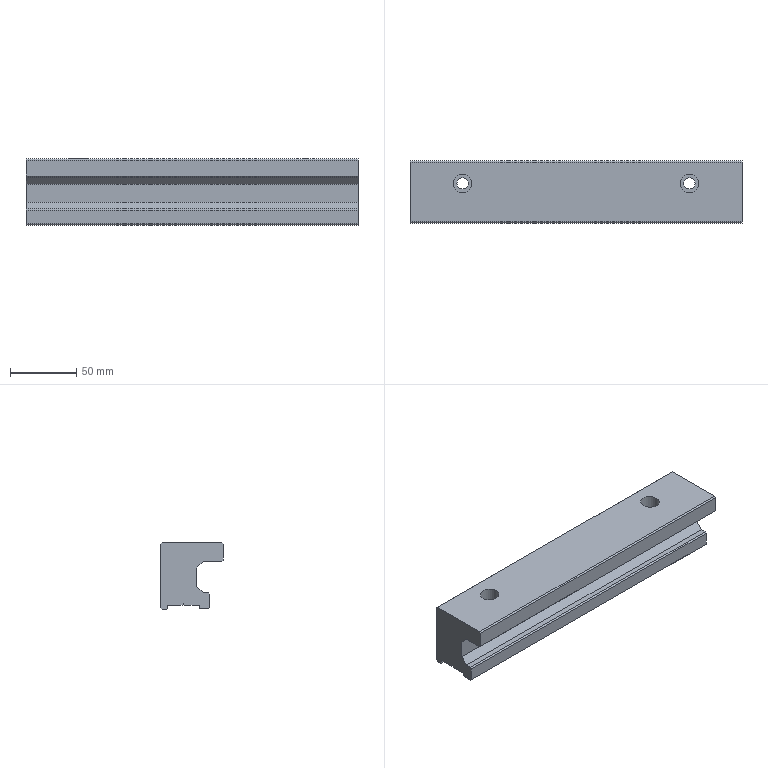Part | NX | features EXTRUDE 3, DATUM_CSYS 2, SKETCH 1 | 1 solid | 37 faces | box 250 x 47 x 50 mm | volume 417029 mm3 | plane 33 | cylinder 4 | commonest cylinder face diameters 8.5 x2 14 x2
STEP:
#1=CARTESIAN_POINT('',(5325.419,6882.013,-47.));
#2=VERTEX_POINT('',#1);
#3=CARTESIAN_POINT('',(5317.158,6882.013,-47.));
#4=VERTEX_POINT('',#3);
#5=CARTESIAN_POINT('',(5321.289,6883.013,-47.));
#6=DIRECTION('',(0.,0.,1.));
#7=DIRECTION('',(1.,0.,0.));
#8=AXIS2_PLACEMENT_3D('',#5,#6,#7);
#9=CIRCLE('',#8,4.25);
#10=EDGE_CURVE('',#2,#4,#9,.F.);
#11=ORIENTED_EDGE('',*,*,#10,.T.);
#12=CARTESIAN_POINT('',(5317.039,6883.013,-46.));
#13=VERTEX_POINT('',#12);
#14=CARTESIAN_POINT('',(5321.289,6883.013,-46.));
#15=DIRECTION('',(0.,-0.7071,0.7071));
#16=DIRECTION('',(0.,0.7071,0.7071));
#17=AXIS2_PLACEMENT_3D('',#14,#15,#16);
#18=ELLIPSE('',#17,6.01,4.25);
#19=EDGE_CURVE('',#4,#13,#18,.F.);
#20=ORIENTED_EDGE('',*,*,#19,.T.);
#21=CARTESIAN_POINT('',(5317.158,6884.013,-47.));
#22=VERTEX_POINT('',#21);
#23=CARTESIAN_POINT('',(5321.289,6883.013,-46.));
#24=DIRECTION('',(0.,0.7071,0.7071));
#25=DIRECTION('',(0.,-0.7071,0.7071));
#26=AXIS2_PLACEMENT_3D('',#23,#24,#25);
#27=ELLIPSE('',#26,6.01,4.25);
#28=EDGE_CURVE('',#13,#22,#27,.F.);
#29=ORIENTED_EDGE('',*,*,#28,.T.);
#30=CARTESIAN_POINT('',(5325.419,6884.013,-47.));
#31=VERTEX_POINT('',#30);
#32=CARTESIAN_POINT('',(5321.289,6883.013,-47.));
#33=DIRECTION('',(0.,0.,1.));
#34=DIRECTION('',(1.,0.,0.));
#35=AXIS2_PLACEMENT_3D('',#32,#33,#34);
#36=CIRCLE('',#35,4.25);
#37=EDGE_CURVE('',#22,#31,#36,.F.);
#38=ORIENTED_EDGE('',*,*,#37,.T.);
#39=CARTESIAN_POINT('',(5325.539,6883.013,-46.));
#40=VERTEX_POINT('',#39);
#41=CARTESIAN_POINT('',(5321.289,6883.013,-46.));
#42=DIRECTION('',(0.,0.7071,0.7071));
#43=DIRECTION('',(0.,-0.7071,0.7071));
#44=AXIS2_PLACEMENT_3D('',#41,#42,#43);
#45=ELLIPSE('',#44,6.01,4.25);
#46=EDGE_CURVE('',#31,#40,#45,.F.);
#47=ORIENTED_EDGE('',*,*,#46,.T.);
#48=CARTESIAN_POINT('',(5321.289,6883.013,-46.));
#49=DIRECTION('',(0.,-0.7071,0.7071));
#50=DIRECTION('',(0.,0.7071,0.7071));
#51=AXIS2_PLACEMENT_3D('',#48,#49,#50);
#52=ELLIPSE('',#51,6.01,4.25);
#53=EDGE_CURVE('',#40,#2,#52,.F.);
#54=ORIENTED_EDGE('',*,*,#53,.T.);
#55=EDGE_LOOP('',(#11,#20,#29,#38,#47,#54));
#56=FACE_BOUND('',#55,.T.);
#57=CARTESIAN_POINT('',(5325.539,6883.013,-12.));
#58=VERTEX_POINT('',#57);
#59=CARTESIAN_POINT('',(5321.289,6883.013,-12.));
#60=DIRECTION('',(0.,0.,1.));
#61=DIRECTION('',(1.,0.,0.));
#62=AXIS2_PLACEMENT_3D('',#59,#60,#61);
#63=CIRCLE('',#62,4.25);
#64=EDGE_CURVE('',#58,#58,#63,.F.);
#65=ORIENTED_EDGE('',*,*,#64,.F.);
#66=EDGE_LOOP('',(#65));
#67=FACE_BOUND('',#66,.T.);
#68=CARTESIAN_POINT('',(5321.289,6883.013,-55000.));
#69=DIRECTION('',(0.,0.,1.));
#70=DIRECTION('',(1.,0.,0.));
#71=AXIS2_PLACEMENT_3D('',#68,#69,#70);
#72=CYLINDRICAL_SURFACE('',#71,4.25);
#73=ADVANCED_FACE('',(#56,#67),#72,.F.);
#74=CARTESIAN_POINT('',(5496.279,6882.013,-47.));
#75=VERTEX_POINT('',#74);
#76=CARTESIAN_POINT('',(5488.017,6882.013,-47.));
#77=VERTEX_POINT('',#76);
#78=CARTESIAN_POINT('',(5492.148,6883.013,-47.));
#79=DIRECTION('',(0.,0.,1.));
#80=DIRECTION('',(1.,0.,0.));
#81=AXIS2_PLACEMENT_3D('',#78,#79,#80);
#82=CIRCLE('',#81,4.25);
#83=EDGE_CURVE('',#75,#77,#82,.F.);
#84=ORIENTED_EDGE('',*,*,#83,.T.);
#85=CARTESIAN_POINT('',(5487.898,6883.013,-46.));
#86=VERTEX_POINT('',#85);
#87=CARTESIAN_POINT('',(5492.148,6883.013,-46.));
#88=DIRECTION('',(0.,-0.7071,0.7071));
#89=DIRECTION('',(0.,0.7071,0.7071));
#90=AXIS2_PLACEMENT_3D('',#87,#88,#89);
#91=ELLIPSE('',#90,6.01,4.25);
#92=EDGE_CURVE('',#77,#86,#91,.F.);
#93=ORIENTED_EDGE('',*,*,#92,.T.);
#94=CARTESIAN_POINT('',(5488.017,6884.013,-47.));
#95=VERTEX_POINT('',#94);
#96=CARTESIAN_POINT('',(5492.148,6883.013,-46.));
#97=DIRECTION('',(0.,0.7071,0.7071));
#98=DIRECTION('',(0.,-0.7071,0.7071));
#99=AXIS2_PLACEMENT_3D('',#96,#97,#98);
#100=ELLIPSE('',#99,6.01,4.25);
#101=EDGE_CURVE('',#86,#95,#100,.F.);
#102=ORIENTED_EDGE('',*,*,#101,.T.);
#103=CARTESIAN_POINT('',(5496.279,6884.013,-47.));
#104=VERTEX_POINT('',#103);
#105=CARTESIAN_POINT('',(5492.148,6883.013,-47.));
#106=DIRECTION('',(0.,0.,1.));
#107=DIRECTION('',(1.,0.,0.));
#108=AXIS2_PLACEMENT_3D('',#105,#106,#107);
#109=CIRCLE('',#108,4.25);
#110=EDGE_CURVE('',#95,#104,#109,.F.);
#111=ORIENTED_EDGE('',*,*,#110,.T.);
#112=CARTESIAN_POINT('',(5496.398,6883.013,-46.));
#113=VERTEX_POINT('',#112);
#114=CARTESIAN_POINT('',(5492.148,6883.013,-46.));
#115=DIRECTION('',(0.,0.7071,0.7071));
#116=DIRECTION('',(0.,-0.7071,0.7071));
#117=AXIS2_PLACEMENT_3D('',#114,#115,#116);
#118=ELLIPSE('',#117,6.01,4.25);
#119=EDGE_CURVE('',#104,#113,#118,.F.);
#120=ORIENTED_EDGE('',*,*,#119,.T.);
#121=CARTESIAN_POINT('',(5492.148,6883.013,-46.));
#122=DIRECTION('',(0.,-0.7071,0.7071));
#123=DIRECTION('',(0.,0.7071,0.7071));
#124=AXIS2_PLACEMENT_3D('',#121,#122,#123);
#125=ELLIPSE('',#124,6.01,4.25);
#126=EDGE_CURVE('',#113,#75,#125,.F.);
#127=ORIENTED_EDGE('',*,*,#126,.T.);
#128=EDGE_LOOP('',(#84,#93,#102,#111,#120,#127));
#129=FACE_BOUND('',#128,.T.);
#130=CARTESIAN_POINT('',(5496.398,6883.013,-12.));
#131=VERTEX_POINT('',#130);
#132=CARTESIAN_POINT('',(5492.148,6883.013,-12.));
#133=DIRECTION('',(0.,0.,1.));
#134=DIRECTION('',(1.,0.,0.));
#135=AXIS2_PLACEMENT_3D('',#132,#133,#134);
#136=CIRCLE('',#135,4.25);
#137=EDGE_CURVE('',#131,#131,#136,.F.);
#138=ORIENTED_EDGE('',*,*,#137,.F.);
#139=EDGE_LOOP('',(#138));
#140=FACE_BOUND('',#139,.T.);
#141=CARTESIAN_POINT('',(5492.148,6883.013,-55000.));
#142=DIRECTION('',(0.,0.,1.));
#143=DIRECTION('',(1.,0.,0.));
#144=AXIS2_PLACEMENT_3D('',#141,#142,#143);
#145=CYLINDRICAL_SURFACE('',#144,4.25);
#146=ADVANCED_FACE('',(#129,#140),#145,.F.);
#147=ORIENTED_EDGE('',*,*,#110,.F.);
#148=CARTESIAN_POINT('',(5281.718,6884.013,-47.));
#149=DIRECTION('',(1.,0.,0.));
#150=VECTOR('',#149,1000.);
#151=LINE('',#148,#150);
#152=EDGE_CURVE('',#31,#95,#151,.T.);
#153=ORIENTED_EDGE('',*,*,#152,.F.);
#154=ORIENTED_EDGE('',*,*,#37,.F.);
#155=CARTESIAN_POINT('',(5281.718,6884.013,-47.));
#156=VERTEX_POINT('',#155);
#157=CARTESIAN_POINT('',(5281.718,6884.013,-47.));
#158=DIRECTION('',(1.,0.,0.));
#159=VECTOR('',#158,1000.);
#160=LINE('',#157,#159);
#161=EDGE_CURVE('',#156,#22,#160,.T.);
#162=ORIENTED_EDGE('',*,*,#161,.F.);
#163=CARTESIAN_POINT('',(5281.718,6895.088,-47.));
#164=VERTEX_POINT('',#163);
#165=CARTESIAN_POINT('',(5281.718,6895.088,-47.));
#166=DIRECTION('',(0.,-1.,0.));
#167=VECTOR('',#166,1000.);
#168=LINE('',#165,#167);
#169=EDGE_CURVE('',#164,#156,#168,.T.);
#170=ORIENTED_EDGE('',*,*,#169,.F.);
#171=CARTESIAN_POINT('',(5531.718,6895.088,-47.));
#172=VERTEX_POINT('',#171);
#173=CARTESIAN_POINT('',(5281.718,6895.088,-47.));
#174=DIRECTION('',(1.,0.,0.));
#175=VECTOR('',#174,1000.);
#176=LINE('',#173,#175);
#177=EDGE_CURVE('',#164,#172,#176,.T.);
#178=ORIENTED_EDGE('',*,*,#177,.T.);
#179=CARTESIAN_POINT('',(5531.718,6884.013,-47.));
#180=VERTEX_POINT('',#179);
#181=CARTESIAN_POINT('',(5531.718,6895.088,-47.));
#182=DIRECTION('',(0.,-1.,0.));
#183=VECTOR('',#182,1000.);
#184=LINE('',#181,#183);
#185=EDGE_CURVE('',#172,#180,#184,.T.);
#186=ORIENTED_EDGE('',*,*,#185,.T.);
#187=CARTESIAN_POINT('',(5281.718,6884.013,-47.));
#188=DIRECTION('',(1.,0.,0.));
#189=VECTOR('',#188,1000.);
#190=LINE('',#187,#189);
#191=EDGE_CURVE('',#104,#180,#190,.T.);
#192=ORIENTED_EDGE('',*,*,#191,.F.);
#193=EDGE_LOOP('',(#147,#153,#154,#162,#170,#178,#186,#192));
#194=FACE_BOUND('',#193,.T.);
#195=CARTESIAN_POINT('',(5281.718,6895.088,-47.));
#196=DIRECTION('',(0.,0.,1.));
#197=DIRECTION('',(1.,0.,0.));
#198=AXIS2_PLACEMENT_3D('',#195,#196,#197);
#199=PLANE('',#198);
#200=ADVANCED_FACE('',(#194),#199,.F.);
#201=ORIENTED_EDGE('',*,*,#101,.F.);
#202=CARTESIAN_POINT('',(5281.718,6883.013,-46.));
#203=DIRECTION('',(1.,0.,0.));
#204=VECTOR('',#203,1000.);
#205=LINE('',#202,#204);
#206=EDGE_CURVE('',#40,#86,#205,.T.);
#207=ORIENTED_EDGE('',*,*,#206,.F.);
#208=ORIENTED_EDGE('',*,*,#46,.F.);
#209=ORIENTED_EDGE('',*,*,#152,.T.);
#210=EDGE_LOOP('',(#201,#207,#208,#209));
#211=FACE_BOUND('',#210,.T.);
#212=CARTESIAN_POINT('',(5281.718,6884.013,-47.));
#213=DIRECTION('',(0.,0.7071,0.7071));
#214=DIRECTION('',(0.,-0.7071,0.7071));
#215=AXIS2_PLACEMENT_3D('',#212,#213,#214);
#216=PLANE('',#215);
#217=ADVANCED_FACE('',(#211),#216,.F.);
#218=ORIENTED_EDGE('',*,*,#119,.F.);
#219=ORIENTED_EDGE('',*,*,#191,.T.);
#220=CARTESIAN_POINT('',(5531.718,6883.013,-46.));
#221=VERTEX_POINT('',#220);
#222=CARTESIAN_POINT('',(5531.718,6884.013,-47.));
#223=DIRECTION('',(0.,-0.7071,0.7071));
#224=VECTOR('',#223,1000.);
#225=LINE('',#222,#224);
#226=EDGE_CURVE('',#180,#221,#225,.T.);
#227=ORIENTED_EDGE('',*,*,#226,.T.);
#228=CARTESIAN_POINT('',(5281.718,6883.013,-46.));
#229=DIRECTION('',(1.,0.,0.));
#230=VECTOR('',#229,1000.);
#231=LINE('',#228,#230);
#232=EDGE_CURVE('',#113,#221,#231,.T.);
#233=ORIENTED_EDGE('',*,*,#232,.F.);
#234=EDGE_LOOP('',(#218,#219,#227,#233));
#235=FACE_BOUND('',#234,.T.);
#236=CARTESIAN_POINT('',(5281.718,6884.013,-47.));
#237=DIRECTION('',(0.,0.7071,0.7071));
#238=DIRECTION('',(0.,-0.7071,0.7071));
#239=AXIS2_PLACEMENT_3D('',#236,#237,#238);
#240=PLANE('',#239);
#241=ADVANCED_FACE('',(#235),#240,.F.);
#242=ORIENTED_EDGE('',*,*,#28,.F.);
#243=CARTESIAN_POINT('',(5281.718,6883.013,-46.));
#244=VERTEX_POINT('',#243);
#245=CARTESIAN_POINT('',(5281.718,6883.013,-46.));
#246=DIRECTION('',(1.,0.,0.));
#247=VECTOR('',#246,1000.);
#248=LINE('',#245,#247);
#249=EDGE_CURVE('',#244,#13,#248,.T.);
#250=ORIENTED_EDGE('',*,*,#249,.F.);
#251=CARTESIAN_POINT('',(5281.718,6884.013,-47.));
#252=DIRECTION('',(0.,-0.7071,0.7071));
#253=VECTOR('',#252,1000.);
#254=LINE('',#251,#253);
#255=EDGE_CURVE('',#156,#244,#254,.T.);
#256=ORIENTED_EDGE('',*,*,#255,.F.);
#257=ORIENTED_EDGE('',*,*,#161,.T.);
#258=EDGE_LOOP('',(#242,#250,#256,#257));
#259=FACE_BOUND('',#258,.T.);
#260=CARTESIAN_POINT('',(5281.718,6884.013,-47.));
#261=DIRECTION('',(0.,0.7071,0.7071));
#262=DIRECTION('',(0.,-0.7071,0.7071));
#263=AXIS2_PLACEMENT_3D('',#260,#261,#262);
#264=PLANE('',#263);
#265=ADVANCED_FACE('',(#259),#264,.F.);
#266=ORIENTED_EDGE('',*,*,#126,.F.);
#267=ORIENTED_EDGE('',*,*,#232,.T.);
#268=CARTESIAN_POINT('',(5531.718,6882.013,-47.));
#269=VERTEX_POINT('',#268);
#270=CARTESIAN_POINT('',(5531.718,6883.013,-46.));
#271=DIRECTION('',(0.,-0.7071,-0.7071));
#272=VECTOR('',#271,1000.);
#273=LINE('',#270,#272);
#274=EDGE_CURVE('',#221,#269,#273,.T.);
#275=ORIENTED_EDGE('',*,*,#274,.T.);
#276=CARTESIAN_POINT('',(5281.718,6882.013,-47.));
#277=DIRECTION('',(1.,0.,0.));
#278=VECTOR('',#277,1000.);
#279=LINE('',#276,#278);
#280=EDGE_CURVE('',#75,#269,#279,.T.);
#281=ORIENTED_EDGE('',*,*,#280,.F.);
#282=EDGE_LOOP('',(#266,#267,#275,#281));
#283=FACE_BOUND('',#282,.T.);
#284=CARTESIAN_POINT('',(5281.718,6883.013,-46.));
#285=DIRECTION('',(0.,-0.7071,0.7071));
#286=DIRECTION('',(0.,-0.7071,-0.7071));
#287=AXIS2_PLACEMENT_3D('',#284,#285,#286);
#288=PLANE('',#287);
#289=ADVANCED_FACE('',(#283),#288,.F.);
#290=ORIENTED_EDGE('',*,*,#92,.F.);
#291=CARTESIAN_POINT('',(5281.718,6882.013,-47.));
#292=DIRECTION('',(1.,0.,0.));
#293=VECTOR('',#292,1000.);
#294=LINE('',#291,#293);
#295=EDGE_CURVE('',#2,#77,#294,.T.);
#296=ORIENTED_EDGE('',*,*,#295,.F.);
#297=ORIENTED_EDGE('',*,*,#53,.F.);
#298=ORIENTED_EDGE('',*,*,#206,.T.);
#299=EDGE_LOOP('',(#290,#296,#297,#298));
#300=FACE_BOUND('',#299,.T.);
#301=CARTESIAN_POINT('',(5281.718,6883.013,-46.));
#302=DIRECTION('',(0.,-0.7071,0.7071));
#303=DIRECTION('',(0.,-0.7071,-0.7071));
#304=AXIS2_PLACEMENT_3D('',#301,#302,#303);
#305=PLANE('',#304);
#306=ADVANCED_FACE('',(#300),#305,.F.);
#307=ORIENTED_EDGE('',*,*,#19,.F.);
#308=CARTESIAN_POINT('',(5281.718,6882.013,-47.));
#309=VERTEX_POINT('',#308);
#310=CARTESIAN_POINT('',(5281.718,6882.013,-47.));
#311=DIRECTION('',(1.,0.,0.));
#312=VECTOR('',#311,1000.);
#313=LINE('',#310,#312);
#314=EDGE_CURVE('',#309,#4,#313,.T.);
#315=ORIENTED_EDGE('',*,*,#314,.F.);
#316=CARTESIAN_POINT('',(5281.718,6883.013,-46.));
#317=DIRECTION('',(0.,-0.7071,-0.7071));
#318=VECTOR('',#317,1000.);
#319=LINE('',#316,#318);
#320=EDGE_CURVE('',#244,#309,#319,.T.);
#321=ORIENTED_EDGE('',*,*,#320,.F.);
#322=ORIENTED_EDGE('',*,*,#249,.T.);
#323=EDGE_LOOP('',(#307,#315,#321,#322));
#324=FACE_BOUND('',#323,.T.);
#325=CARTESIAN_POINT('',(5281.718,6883.013,-46.));
#326=DIRECTION('',(0.,-0.7071,0.7071));
#327=DIRECTION('',(0.,-0.7071,-0.7071));
#328=AXIS2_PLACEMENT_3D('',#325,#326,#327);
#329=PLANE('',#328);
#330=ADVANCED_FACE('',(#324),#329,.F.);
#331=ORIENTED_EDGE('',*,*,#83,.F.);
#332=ORIENTED_EDGE('',*,*,#280,.T.);
#333=CARTESIAN_POINT('',(5531.718,6870.938,-47.));
#334=VERTEX_POINT('',#333);
#335=CARTESIAN_POINT('',(5531.718,6882.013,-47.));
#336=DIRECTION('',(0.,-1.,0.));
#337=VECTOR('',#336,1000.);
#338=LINE('',#335,#337);
#339=EDGE_CURVE('',#269,#334,#338,.T.);
#340=ORIENTED_EDGE('',*,*,#339,.T.);
#341=CARTESIAN_POINT('',(5281.718,6870.938,-47.));
#342=VERTEX_POINT('',#341);
#343=CARTESIAN_POINT('',(5281.718,6870.938,-47.));
#344=DIRECTION('',(1.,0.,0.));
#345=VECTOR('',#344,1000.);
#346=LINE('',#343,#345);
#347=EDGE_CURVE('',#342,#334,#346,.T.);
#348=ORIENTED_EDGE('',*,*,#347,.F.);
#349=CARTESIAN_POINT('',(5281.718,6882.013,-47.));
#350=DIRECTION('',(0.,-1.,0.));
#351=VECTOR('',#350,1000.);
#352=LINE('',#349,#351);
#353=EDGE_CURVE('',#309,#342,#352,.T.);
#354=ORIENTED_EDGE('',*,*,#353,.F.);
#355=ORIENTED_EDGE('',*,*,#314,.T.);
#356=ORIENTED_EDGE('',*,*,#10,.F.);
#357=ORIENTED_EDGE('',*,*,#295,.T.);
#358=EDGE_LOOP('',(#331,#332,#340,#348,#354,#355,#356,#357));
#359=FACE_BOUND('',#358,.T.);
#360=CARTESIAN_POINT('',(5281.718,6882.013,-47.));
#361=DIRECTION('',(0.,0.,1.));
#362=DIRECTION('',(1.,0.,0.));
#363=AXIS2_PLACEMENT_3D('',#360,#361,#362);
#364=PLANE('',#363);
#365=ADVANCED_FACE('',(#359),#364,.F.);
#366=CARTESIAN_POINT('',(5531.718,6899.013,0.));
#367=VERTEX_POINT('',#366);
#368=CARTESIAN_POINT('',(5531.718,6900.013,-1.));
#369=VERTEX_POINT('',#368);
#370=CARTESIAN_POINT('',(5531.718,6899.013,0.));
#371=DIRECTION('',(0.,0.7071,-0.7071));
#372=VECTOR('',#371,1000.);
#373=LINE('',#370,#372);
#374=EDGE_CURVE('',#367,#369,#373,.T.);
#375=ORIENTED_EDGE('',*,*,#374,.T.);
#376=CARTESIAN_POINT('',(5281.718,6900.013,-1.));
#377=VERTEX_POINT('',#376);
#378=CARTESIAN_POINT('',(5281.718,6900.013,-1.));
#379=DIRECTION('',(1.,0.,0.));
#380=VECTOR('',#379,1000.);
#381=LINE('',#378,#380);
#382=EDGE_CURVE('',#377,#369,#381,.T.);
#383=ORIENTED_EDGE('',*,*,#382,.F.);
#384=CARTESIAN_POINT('',(5281.718,6899.013,0.));
#385=VERTEX_POINT('',#384);
#386=CARTESIAN_POINT('',(5281.718,6899.013,0.));
#387=DIRECTION('',(0.,0.7071,-0.7071));
#388=VECTOR('',#387,1000.);
#389=LINE('',#386,#388);
#390=EDGE_CURVE('',#385,#377,#389,.T.);
#391=ORIENTED_EDGE('',*,*,#390,.F.);
#392=CARTESIAN_POINT('',(5281.718,6899.013,0.));
#393=DIRECTION('',(1.,0.,0.));
#394=VECTOR('',#393,1000.);
#395=LINE('',#392,#394);
#396=EDGE_CURVE('',#385,#367,#395,.T.);
#397=ORIENTED_EDGE('',*,*,#396,.T.);
#398=EDGE_LOOP('',(#375,#383,#391,#397));
#399=FACE_BOUND('',#398,.T.);
#400=CARTESIAN_POINT('',(5281.718,6899.013,0.));
#401=DIRECTION('',(0.,-0.7071,-0.7071));
#402=DIRECTION('',(0.,0.7071,-0.7071));
#403=AXIS2_PLACEMENT_3D('',#400,#401,#402);
#404=PLANE('',#403);
#405=ADVANCED_FACE('',(#399),#404,.F.);
#406=CARTESIAN_POINT('',(5531.718,6900.013,-49.));
#407=VERTEX_POINT('',#406);
#408=CARTESIAN_POINT('',(5531.718,6900.013,-1.));
#409=DIRECTION('',(0.,0.,-1.));
#410=VECTOR('',#409,1000.);
#411=LINE('',#408,#410);
#412=EDGE_CURVE('',#369,#407,#411,.T.);
#413=ORIENTED_EDGE('',*,*,#412,.T.);
#414=CARTESIAN_POINT('',(5281.718,6900.013,-49.));
#415=VERTEX_POINT('',#414);
#416=CARTESIAN_POINT('',(5281.718,6900.013,-49.));
#417=DIRECTION('',(1.,0.,0.));
#418=VECTOR('',#417,1000.);
#419=LINE('',#416,#418);
#420=EDGE_CURVE('',#415,#407,#419,.T.);
#421=ORIENTED_EDGE('',*,*,#420,.F.);
#422=CARTESIAN_POINT('',(5281.718,6900.013,-1.));
#423=DIRECTION('',(0.,0.,-1.));
#424=VECTOR('',#423,1000.);
#425=LINE('',#422,#424);
#426=EDGE_CURVE('',#377,#415,#425,.T.);
#427=ORIENTED_EDGE('',*,*,#426,.F.);
#428=ORIENTED_EDGE('',*,*,#382,.T.);
#429=EDGE_LOOP('',(#413,#421,#427,#428));
#430=FACE_BOUND('',#429,.T.);
#431=CARTESIAN_POINT('',(5281.718,6900.013,-1.));
#432=DIRECTION('',(0.,-1.,0.));
#433=DIRECTION('',(0.,0.,-1.));
#434=AXIS2_PLACEMENT_3D('',#431,#432,#433);
#435=PLANE('',#434);
#436=ADVANCED_FACE('',(#430),#435,.F.);
#437=CARTESIAN_POINT('',(5531.718,6899.013,-50.));
#438=VERTEX_POINT('',#437);
#439=CARTESIAN_POINT('',(5531.718,6900.013,-49.));
#440=DIRECTION('',(0.,-0.7071,-0.7071));
#441=VECTOR('',#440,1000.);
#442=LINE('',#439,#441);
#443=EDGE_CURVE('',#407,#438,#442,.T.);
#444=ORIENTED_EDGE('',*,*,#443,.T.);
#445=CARTESIAN_POINT('',(5281.718,6899.013,-50.));
#446=VERTEX_POINT('',#445);
#447=CARTESIAN_POINT('',(5281.718,6899.013,-50.));
#448=DIRECTION('',(1.,0.,0.));
#449=VECTOR('',#448,1000.);
#450=LINE('',#447,#449);
#451=EDGE_CURVE('',#446,#438,#450,.T.);
#452=ORIENTED_EDGE('',*,*,#451,.F.);
#453=CARTESIAN_POINT('',(5281.718,6900.013,-49.));
#454=DIRECTION('',(0.,-0.7071,-0.7071));
#455=VECTOR('',#454,1000.);
#456=LINE('',#453,#455);
#457=EDGE_CURVE('',#415,#446,#456,.T.);
#458=ORIENTED_EDGE('',*,*,#457,.F.);
#459=ORIENTED_EDGE('',*,*,#420,.T.);
#460=EDGE_LOOP('',(#444,#452,#458,#459));
#461=FACE_BOUND('',#460,.T.);
#462=CARTESIAN_POINT('',(5281.718,6900.013,-49.));
#463=DIRECTION('',(0.,-0.7071,0.7071));
#464=DIRECTION('',(0.,-0.7071,-0.7071));
#465=AXIS2_PLACEMENT_3D('',#462,#463,#464);
#466=PLANE('',#465);
#467=ADVANCED_FACE('',(#461),#466,.F.);
#468=CARTESIAN_POINT('',(5531.718,6895.588,-50.));
#469=VERTEX_POINT('',#468);
#470=CARTESIAN_POINT('',(5531.718,6899.013,-50.));
#471=DIRECTION('',(0.,-1.,0.));
#472=VECTOR('',#471,1000.);
#473=LINE('',#470,#472);
#474=EDGE_CURVE('',#438,#469,#473,.T.);
#475=ORIENTED_EDGE('',*,*,#474,.T.);
#476=CARTESIAN_POINT('',(5281.718,6895.588,-50.));
#477=VERTEX_POINT('',#476);
#478=CARTESIAN_POINT('',(5281.718,6895.588,-50.));
#479=DIRECTION('',(1.,0.,0.));
#480=VECTOR('',#479,1000.);
#481=LINE('',#478,#480);
#482=EDGE_CURVE('',#477,#469,#481,.T.);
#483=ORIENTED_EDGE('',*,*,#482,.F.);
#484=CARTESIAN_POINT('',(5281.718,6899.013,-50.));
#485=DIRECTION('',(0.,-1.,0.));
#486=VECTOR('',#485,1000.);
#487=LINE('',#484,#486);
#488=EDGE_CURVE('',#446,#477,#487,.T.);
#489=ORIENTED_EDGE('',*,*,#488,.F.);
#490=ORIENTED_EDGE('',*,*,#451,.T.);
#491=EDGE_LOOP('',(#475,#483,#489,#490));
#492=FACE_BOUND('',#491,.T.);
#493=CARTESIAN_POINT('',(5281.718,6899.013,-50.));
#494=DIRECTION('',(0.,0.,1.));
#495=DIRECTION('',(1.,0.,0.));
#496=AXIS2_PLACEMENT_3D('',#493,#494,#495);
#497=PLANE('',#496);
#498=ADVANCED_FACE('',(#492),#497,.F.);
#499=CARTESIAN_POINT('',(5531.718,6895.088,-49.5));
#500=VERTEX_POINT('',#499);
#501=CARTESIAN_POINT('',(5531.718,6895.588,-50.));
#502=DIRECTION('',(0.,-0.7071,0.7071));
#503=VECTOR('',#502,1000.);
#504=LINE('',#501,#503);
#505=EDGE_CURVE('',#469,#500,#504,.T.);
#506=ORIENTED_EDGE('',*,*,#505,.T.);
#507=CARTESIAN_POINT('',(5281.718,6895.088,-49.5));
#508=VERTEX_POINT('',#507);
#509=CARTESIAN_POINT('',(5281.718,6895.088,-49.5));
#510=DIRECTION('',(1.,0.,0.));
#511=VECTOR('',#510,1000.);
#512=LINE('',#509,#511);
#513=EDGE_CURVE('',#508,#500,#512,.T.);
#514=ORIENTED_EDGE('',*,*,#513,.F.);
#515=CARTESIAN_POINT('',(5281.718,6895.588,-50.));
#516=DIRECTION('',(0.,-0.7071,0.7071));
#517=VECTOR('',#516,1000.);
#518=LINE('',#515,#517);
#519=EDGE_CURVE('',#477,#508,#518,.T.);
#520=ORIENTED_EDGE('',*,*,#519,.F.);
#521=ORIENTED_EDGE('',*,*,#482,.T.);
#522=EDGE_LOOP('',(#506,#514,#520,#521));
#523=FACE_BOUND('',#522,.T.);
#524=CARTESIAN_POINT('',(5281.718,6895.588,-50.));
#525=DIRECTION('',(0.,0.7071,0.7071));
#526=DIRECTION('',(0.,-0.7071,0.7071));
#527=AXIS2_PLACEMENT_3D('',#524,#525,#526);
#528=PLANE('',#527);
#529=ADVANCED_FACE('',(#523),#528,.F.);
#530=CARTESIAN_POINT('',(5531.718,6895.088,-49.5));
#531=DIRECTION('',(0.,0.,1.));
#532=VECTOR('',#531,1000.);
#533=LINE('',#530,#532);
#534=EDGE_CURVE('',#500,#172,#533,.T.);
#535=ORIENTED_EDGE('',*,*,#534,.T.);
#536=ORIENTED_EDGE('',*,*,#177,.F.);
#537=CARTESIAN_POINT('',(5281.718,6895.088,-49.5));
#538=DIRECTION('',(0.,0.,1.));
#539=VECTOR('',#538,1000.);
#540=LINE('',#537,#539);
#541=EDGE_CURVE('',#508,#164,#540,.T.);
#542=ORIENTED_EDGE('',*,*,#541,.F.);
#543=ORIENTED_EDGE('',*,*,#513,.T.);
#544=EDGE_LOOP('',(#535,#536,#542,#543));
#545=FACE_BOUND('',#544,.T.);
#546=CARTESIAN_POINT('',(5281.718,6895.088,-49.5));
#547=DIRECTION('',(0.,1.,0.));
#548=DIRECTION('',(0.,0.,1.));
#549=AXIS2_PLACEMENT_3D('',#546,#547,#548);
#550=PLANE('',#549);
#551=ADVANCED_FACE('',(#545),#550,.F.);
#552=CARTESIAN_POINT('',(5531.718,6870.938,-49.3));
#553=VERTEX_POINT('',#552);
#554=CARTESIAN_POINT('',(5531.718,6870.938,-47.));
#555=DIRECTION('',(0.,0.,-1.));
#556=VECTOR('',#555,1000.);
#557=LINE('',#554,#556);
#558=EDGE_CURVE('',#334,#553,#557,.T.);
#559=ORIENTED_EDGE('',*,*,#558,.T.);
#560=CARTESIAN_POINT('',(5281.718,6870.938,-49.3));
#561=VERTEX_POINT('',#560);
#562=CARTESIAN_POINT('',(5281.718,6870.938,-49.3));
#563=DIRECTION('',(1.,0.,0.));
#564=VECTOR('',#563,1000.);
#565=LINE('',#562,#564);
#566=EDGE_CURVE('',#561,#553,#565,.T.);
#567=ORIENTED_EDGE('',*,*,#566,.F.);
#568=CARTESIAN_POINT('',(5281.718,6870.938,-47.));
#569=DIRECTION('',(0.,0.,-1.));
#570=VECTOR('',#569,1000.);
#571=LINE('',#568,#570);
#572=EDGE_CURVE('',#342,#561,#571,.T.);
#573=ORIENTED_EDGE('',*,*,#572,.F.);
#574=ORIENTED_EDGE('',*,*,#347,.T.);
#575=EDGE_LOOP('',(#559,#567,#573,#574));
#576=FACE_BOUND('',#575,.T.);
#577=CARTESIAN_POINT('',(5281.718,6870.938,-47.));
#578=DIRECTION('',(0.,-1.,0.));
#579=DIRECTION('',(0.,0.,-1.));
#580=AXIS2_PLACEMENT_3D('',#577,#578,#579);
#581=PLANE('',#580);
#582=ADVANCED_FACE('',(#576),#581,.F.);
#583=CARTESIAN_POINT('',(5531.718,6870.438,-49.8));
#584=VERTEX_POINT('',#583);
#585=CARTESIAN_POINT('',(5531.718,6870.938,-49.3));
#586=DIRECTION('',(0.,-0.7071,-0.7071));
#587=VECTOR('',#586,1000.);
#588=LINE('',#585,#587);
#589=EDGE_CURVE('',#553,#584,#588,.T.);
#590=ORIENTED_EDGE('',*,*,#589,.T.);
#591=CARTESIAN_POINT('',(5281.718,6870.438,-49.8));
#592=VERTEX_POINT('',#591);
#593=CARTESIAN_POINT('',(5281.718,6870.438,-49.8));
#594=DIRECTION('',(1.,0.,0.));
#595=VECTOR('',#594,1000.);
#596=LINE('',#593,#595);
#597=EDGE_CURVE('',#592,#584,#596,.T.);
#598=ORIENTED_EDGE('',*,*,#597,.F.);
#599=CARTESIAN_POINT('',(5281.718,6870.938,-49.3));
#600=DIRECTION('',(0.,-0.7071,-0.7071));
#601=VECTOR('',#600,1000.);
#602=LINE('',#599,#601);
#603=EDGE_CURVE('',#561,#592,#602,.T.);
#604=ORIENTED_EDGE('',*,*,#603,.F.);
#605=ORIENTED_EDGE('',*,*,#566,.T.);
#606=EDGE_LOOP('',(#590,#598,#604,#605));
#607=FACE_BOUND('',#606,.T.);
#608=CARTESIAN_POINT('',(5281.718,6870.938,-49.3));
#609=DIRECTION('',(0.,-0.7071,0.7071));
#610=DIRECTION('',(0.,-0.7071,-0.7071));
#611=AXIS2_PLACEMENT_3D('',#608,#609,#610);
#612=PLANE('',#611);
#613=ADVANCED_FACE('',(#607),#612,.F.);
#614=CARTESIAN_POINT('',(5531.718,6864.013,-49.8));
#615=VERTEX_POINT('',#614);
#616=CARTESIAN_POINT('',(5531.718,6870.438,-49.8));
#617=DIRECTION('',(0.,-1.,0.));
#618=VECTOR('',#617,1000.);
#619=LINE('',#616,#618);
#620=EDGE_CURVE('',#584,#615,#619,.T.);
#621=ORIENTED_EDGE('',*,*,#620,.T.);
#622=CARTESIAN_POINT('',(5281.718,6864.013,-49.8));
#623=VERTEX_POINT('',#622);
#624=CARTESIAN_POINT('',(5281.718,6864.013,-49.8));
#625=DIRECTION('',(1.,0.,0.));
#626=VECTOR('',#625,1000.);
#627=LINE('',#624,#626);
#628=EDGE_CURVE('',#623,#615,#627,.T.);
#629=ORIENTED_EDGE('',*,*,#628,.F.);
#630=CARTESIAN_POINT('',(5281.718,6870.438,-49.8));
#631=DIRECTION('',(0.,-1.,0.));
#632=VECTOR('',#631,1000.);
#633=LINE('',#630,#632);
#634=EDGE_CURVE('',#592,#623,#633,.T.);
#635=ORIENTED_EDGE('',*,*,#634,.F.);
#636=ORIENTED_EDGE('',*,*,#597,.T.);
#637=EDGE_LOOP('',(#621,#629,#635,#636));
#638=FACE_BOUND('',#637,.T.);
#639=CARTESIAN_POINT('',(5281.718,6870.438,-49.8));
#640=DIRECTION('',(0.,0.,1.));
#641=DIRECTION('',(1.,0.,0.));
#642=AXIS2_PLACEMENT_3D('',#639,#640,#641);
#643=PLANE('',#642);
#644=ADVANCED_FACE('',(#638),#643,.F.);
#645=CARTESIAN_POINT('',(5531.718,6863.013,-48.8));
#646=VERTEX_POINT('',#645);
#647=CARTESIAN_POINT('',(5531.718,6864.013,-49.8));
#648=DIRECTION('',(0.,-0.7071,0.7071));
#649=VECTOR('',#648,1000.);
#650=LINE('',#647,#649);
#651=EDGE_CURVE('',#615,#646,#650,.T.);
#652=ORIENTED_EDGE('',*,*,#651,.T.);
#653=CARTESIAN_POINT('',(5281.718,6863.013,-48.8));
#654=VERTEX_POINT('',#653);
#655=CARTESIAN_POINT('',(5281.718,6863.013,-48.8));
#656=DIRECTION('',(1.,0.,0.));
#657=VECTOR('',#656,1000.);
#658=LINE('',#655,#657);
#659=EDGE_CURVE('',#654,#646,#658,.T.);
#660=ORIENTED_EDGE('',*,*,#659,.F.);
#661=CARTESIAN_POINT('',(5281.718,6864.013,-49.8));
#662=DIRECTION('',(0.,-0.7071,0.7071));
#663=VECTOR('',#662,1000.);
#664=LINE('',#661,#663);
#665=EDGE_CURVE('',#623,#654,#664,.T.);
#666=ORIENTED_EDGE('',*,*,#665,.F.);
#667=ORIENTED_EDGE('',*,*,#628,.T.);
#668=EDGE_LOOP('',(#652,#660,#666,#667));
#669=FACE_BOUND('',#668,.T.);
#670=CARTESIAN_POINT('',(5281.718,6864.013,-49.8));
#671=DIRECTION('',(0.,0.7071,0.7071));
#672=DIRECTION('',(0.,-0.7071,0.7071));
#673=AXIS2_PLACEMENT_3D('',#670,#671,#672);
#674=PLANE('',#673);
#675=ADVANCED_FACE('',(#669),#674,.F.);
#676=CARTESIAN_POINT('',(5531.718,6863.013,-38.8));
#677=VERTEX_POINT('',#676);
#678=CARTESIAN_POINT('',(5531.718,6863.013,-48.8));
#679=DIRECTION('',(0.,0.,1.));
#680=VECTOR('',#679,1000.);
#681=LINE('',#678,#680);
#682=EDGE_CURVE('',#646,#677,#681,.T.);
#683=ORIENTED_EDGE('',*,*,#682,.T.);
#684=CARTESIAN_POINT('',(5281.718,6863.013,-38.8));
#685=VERTEX_POINT('',#684);
#686=CARTESIAN_POINT('',(5281.718,6863.013,-38.8));
#687=DIRECTION('',(1.,0.,0.));
#688=VECTOR('',#687,1000.);
#689=LINE('',#686,#688);
#690=EDGE_CURVE('',#685,#677,#689,.T.);
#691=ORIENTED_EDGE('',*,*,#690,.F.);
#692=CARTESIAN_POINT('',(5281.718,6863.013,-48.8));
#693=DIRECTION('',(0.,0.,1.));
#694=VECTOR('',#693,1000.);
#695=LINE('',#692,#694);
#696=EDGE_CURVE('',#654,#685,#695,.T.);
#697=ORIENTED_EDGE('',*,*,#696,.F.);
#698=ORIENTED_EDGE('',*,*,#659,.T.);
#699=EDGE_LOOP('',(#683,#691,#697,#698));
#700=FACE_BOUND('',#699,.T.);
#701=CARTESIAN_POINT('',(5281.718,6863.013,-48.8));
#702=DIRECTION('',(0.,1.,0.));
#703=DIRECTION('',(0.,0.,1.));
#704=AXIS2_PLACEMENT_3D('',#701,#702,#703);
#705=PLANE('',#704);
#706=ADVANCED_FACE('',(#700),#705,.F.);
#707=CARTESIAN_POINT('',(5531.718,6864.013,-37.8));
#708=VERTEX_POINT('',#707);
#709=CARTESIAN_POINT('',(5531.718,6863.013,-38.8));
#710=DIRECTION('',(0.,0.7071,0.7071));
#711=VECTOR('',#710,1000.);
#712=LINE('',#709,#711);
#713=EDGE_CURVE('',#677,#708,#712,.T.);
#714=ORIENTED_EDGE('',*,*,#713,.T.);
#715=CARTESIAN_POINT('',(5281.718,6864.013,-37.8));
#716=VERTEX_POINT('',#715);
#717=CARTESIAN_POINT('',(5281.718,6864.013,-37.8));
#718=DIRECTION('',(1.,0.,0.));
#719=VECTOR('',#718,1000.);
#720=LINE('',#717,#719);
#721=EDGE_CURVE('',#716,#708,#720,.T.);
#722=ORIENTED_EDGE('',*,*,#721,.F.);
#723=CARTESIAN_POINT('',(5281.718,6863.013,-38.8));
#724=DIRECTION('',(0.,0.7071,0.7071));
#725=VECTOR('',#724,1000.);
#726=LINE('',#723,#725);
#727=EDGE_CURVE('',#685,#716,#726,.T.);
#728=ORIENTED_EDGE('',*,*,#727,.F.);
#729=ORIENTED_EDGE('',*,*,#690,.T.);
#730=EDGE_LOOP('',(#714,#722,#728,#729));
#731=FACE_BOUND('',#730,.T.);
#732=CARTESIAN_POINT('',(5281.718,6863.013,-38.8));
#733=DIRECTION('',(0.,0.7071,-0.7071));
#734=DIRECTION('',(0.,0.7071,0.7071));
#735=AXIS2_PLACEMENT_3D('',#732,#733,#734);
#736=PLANE('',#735);
#737=ADVANCED_FACE('',(#731),#736,.F.);
#738=CARTESIAN_POINT('',(5531.718,6868.013,-37.8));
#739=VERTEX_POINT('',#738);
#740=CARTESIAN_POINT('',(5531.718,6864.013,-37.8));
#741=DIRECTION('',(0.,1.,0.));
#742=VECTOR('',#741,1000.);
#743=LINE('',#740,#742);
#744=EDGE_CURVE('',#708,#739,#743,.T.);
#745=ORIENTED_EDGE('',*,*,#744,.T.);
#746=CARTESIAN_POINT('',(5281.718,6868.013,-37.8));
#747=VERTEX_POINT('',#746);
#748=CARTESIAN_POINT('',(5281.718,6868.013,-37.8));
#749=DIRECTION('',(1.,0.,0.));
#750=VECTOR('',#749,1000.);
#751=LINE('',#748,#750);
#752=EDGE_CURVE('',#747,#739,#751,.T.);
#753=ORIENTED_EDGE('',*,*,#752,.F.);
#754=CARTESIAN_POINT('',(5281.718,6864.013,-37.8));
#755=DIRECTION('',(0.,1.,0.));
#756=VECTOR('',#755,1000.);
#757=LINE('',#754,#756);
#758=EDGE_CURVE('',#716,#747,#757,.T.);
#759=ORIENTED_EDGE('',*,*,#758,.F.);
#760=ORIENTED_EDGE('',*,*,#721,.T.);
#761=EDGE_LOOP('',(#745,#753,#759,#760));
#762=FACE_BOUND('',#761,.T.);
#763=CARTESIAN_POINT('',(5281.718,6864.013,-37.8));
#764=DIRECTION('',(0.,0.,-1.));
#765=DIRECTION('',(-1.,0.,0.));
#766=AXIS2_PLACEMENT_3D('',#763,#764,#765);
#767=PLANE('',#766);
#768=ADVANCED_FACE('',(#762),#767,.F.);
#769=CARTESIAN_POINT('',(5531.718,6873.013,-32.8));
#770=VERTEX_POINT('',#769);
#771=CARTESIAN_POINT('',(5531.718,6868.013,-37.8));
#772=DIRECTION('',(0.,0.7071,0.7071));
#773=VECTOR('',#772,1000.);
#774=LINE('',#771,#773);
#775=EDGE_CURVE('',#739,#770,#774,.T.);
#776=ORIENTED_EDGE('',*,*,#775,.T.);
#777=CARTESIAN_POINT('',(5281.718,6873.013,-32.8));
#778=VERTEX_POINT('',#777);
#779=CARTESIAN_POINT('',(5281.718,6873.013,-32.8));
#780=DIRECTION('',(1.,0.,0.));
#781=VECTOR('',#780,1000.);
#782=LINE('',#779,#781);
#783=EDGE_CURVE('',#778,#770,#782,.T.);
#784=ORIENTED_EDGE('',*,*,#783,.F.);
#785=CARTESIAN_POINT('',(5281.718,6868.013,-37.8));
#786=DIRECTION('',(0.,0.7071,0.7071));
#787=VECTOR('',#786,1000.);
#788=LINE('',#785,#787);
#789=EDGE_CURVE('',#747,#778,#788,.T.);
#790=ORIENTED_EDGE('',*,*,#789,.F.);
#791=ORIENTED_EDGE('',*,*,#752,.T.);
#792=EDGE_LOOP('',(#776,#784,#790,#791));
#793=FACE_BOUND('',#792,.T.);
#794=CARTESIAN_POINT('',(5281.718,6868.013,-37.8));
#795=DIRECTION('',(0.,0.7071,-0.7071));
#796=DIRECTION('',(0.,0.7071,0.7071));
#797=AXIS2_PLACEMENT_3D('',#794,#795,#796);
#798=PLANE('',#797);
#799=ADVANCED_FACE('',(#793),#798,.F.);
#800=CARTESIAN_POINT('',(5531.718,6873.013,-19.));
#801=VERTEX_POINT('',#800);
#802=CARTESIAN_POINT('',(5531.718,6873.013,-32.8));
#803=DIRECTION('',(0.,0.,1.));
#804=VECTOR('',#803,1000.);
#805=LINE('',#802,#804);
#806=EDGE_CURVE('',#770,#801,#805,.T.);
#807=ORIENTED_EDGE('',*,*,#806,.T.);
#808=CARTESIAN_POINT('',(5281.718,6873.013,-19.));
#809=VERTEX_POINT('',#808);
#810=CARTESIAN_POINT('',(5281.718,6873.013,-19.));
#811=DIRECTION('',(1.,0.,0.));
#812=VECTOR('',#811,1000.);
#813=LINE('',#810,#812);
#814=EDGE_CURVE('',#809,#801,#813,.T.);
#815=ORIENTED_EDGE('',*,*,#814,.F.);
#816=CARTESIAN_POINT('',(5281.718,6873.013,-32.8));
#817=DIRECTION('',(0.,0.,1.));
#818=VECTOR('',#817,1000.);
#819=LINE('',#816,#818);
#820=EDGE_CURVE('',#778,#809,#819,.T.);
#821=ORIENTED_EDGE('',*,*,#820,.F.);
#822=ORIENTED_EDGE('',*,*,#783,.T.);
#823=EDGE_LOOP('',(#807,#815,#821,#822));
#824=FACE_BOUND('',#823,.T.);
#825=CARTESIAN_POINT('',(5281.718,6873.013,-32.8));
#826=DIRECTION('',(0.,1.,0.));
#827=DIRECTION('',(0.,0.,1.));
#828=AXIS2_PLACEMENT_3D('',#825,#826,#827);
#829=PLANE('',#828);
#830=ADVANCED_FACE('',(#824),#829,.F.);
#831=CARTESIAN_POINT('',(5531.718,6868.013,-14.));
#832=VERTEX_POINT('',#831);
#833=CARTESIAN_POINT('',(5531.718,6873.013,-19.));
#834=DIRECTION('',(0.,-0.7071,0.7071));
#835=VECTOR('',#834,1000.);
#836=LINE('',#833,#835);
#837=EDGE_CURVE('',#801,#832,#836,.T.);
#838=ORIENTED_EDGE('',*,*,#837,.T.);
#839=CARTESIAN_POINT('',(5281.718,6868.013,-14.));
#840=VERTEX_POINT('',#839);
#841=CARTESIAN_POINT('',(5281.718,6868.013,-14.));
#842=DIRECTION('',(1.,0.,0.));
#843=VECTOR('',#842,1000.);
#844=LINE('',#841,#843);
#845=EDGE_CURVE('',#840,#832,#844,.T.);
#846=ORIENTED_EDGE('',*,*,#845,.F.);
#847=CARTESIAN_POINT('',(5281.718,6873.013,-19.));
#848=DIRECTION('',(0.,-0.7071,0.7071));
#849=VECTOR('',#848,1000.);
#850=LINE('',#847,#849);
#851=EDGE_CURVE('',#809,#840,#850,.T.);
#852=ORIENTED_EDGE('',*,*,#851,.F.);
#853=ORIENTED_EDGE('',*,*,#814,.T.);
#854=EDGE_LOOP('',(#838,#846,#852,#853));
#855=FACE_BOUND('',#854,.T.);
#856=CARTESIAN_POINT('',(5281.718,6873.013,-19.));
#857=DIRECTION('',(0.,0.7071,0.7071));
#858=DIRECTION('',(0.,-0.7071,0.7071));
#859=AXIS2_PLACEMENT_3D('',#856,#857,#858);
#860=PLANE('',#859);
#861=ADVANCED_FACE('',(#855),#860,.F.);
#862=CARTESIAN_POINT('',(5531.718,6854.013,-14.));
#863=VERTEX_POINT('',#862);
#864=CARTESIAN_POINT('',(5531.718,6868.013,-14.));
#865=DIRECTION('',(0.,-1.,0.));
#866=VECTOR('',#865,1000.);
#867=LINE('',#864,#866);
#868=EDGE_CURVE('',#832,#863,#867,.T.);
#869=ORIENTED_EDGE('',*,*,#868,.T.);
#870=CARTESIAN_POINT('',(5281.718,6854.013,-14.));
#871=VERTEX_POINT('',#870);
#872=CARTESIAN_POINT('',(5281.718,6854.013,-14.));
#873=DIRECTION('',(1.,0.,0.));
#874=VECTOR('',#873,1000.);
#875=LINE('',#872,#874);
#876=EDGE_CURVE('',#871,#863,#875,.T.);
#877=ORIENTED_EDGE('',*,*,#876,.F.);
#878=CARTESIAN_POINT('',(5281.718,6868.013,-14.));
#879=DIRECTION('',(0.,-1.,0.));
#880=VECTOR('',#879,1000.);
#881=LINE('',#878,#880);
#882=EDGE_CURVE('',#840,#871,#881,.T.);
#883=ORIENTED_EDGE('',*,*,#882,.F.);
#884=ORIENTED_EDGE('',*,*,#845,.T.);
#885=EDGE_LOOP('',(#869,#877,#883,#884));
#886=FACE_BOUND('',#885,.T.);
#887=CARTESIAN_POINT('',(5281.718,6868.013,-14.));
#888=DIRECTION('',(0.,0.,1.));
#889=DIRECTION('',(1.,0.,0.));
#890=AXIS2_PLACEMENT_3D('',#887,#888,#889);
#891=PLANE('',#890);
#892=ADVANCED_FACE('',(#886),#891,.F.);
#893=CARTESIAN_POINT('',(5531.718,6853.013,-13.));
#894=VERTEX_POINT('',#893);
#895=CARTESIAN_POINT('',(5531.718,6854.013,-14.));
#896=DIRECTION('',(0.,-0.7071,0.7071));
#897=VECTOR('',#896,1000.);
#898=LINE('',#895,#897);
#899=EDGE_CURVE('',#863,#894,#898,.T.);
#900=ORIENTED_EDGE('',*,*,#899,.T.);
#901=CARTESIAN_POINT('',(5281.718,6853.013,-13.));
#902=VERTEX_POINT('',#901);
#903=CARTESIAN_POINT('',(5281.718,6853.013,-13.));
#904=DIRECTION('',(1.,0.,0.));
#905=VECTOR('',#904,1000.);
#906=LINE('',#903,#905);
#907=EDGE_CURVE('',#902,#894,#906,.T.);
#908=ORIENTED_EDGE('',*,*,#907,.F.);
#909=CARTESIAN_POINT('',(5281.718,6854.013,-14.));
#910=DIRECTION('',(0.,-0.7071,0.7071));
#911=VECTOR('',#910,1000.);
#912=LINE('',#909,#911);
#913=EDGE_CURVE('',#871,#902,#912,.T.);
#914=ORIENTED_EDGE('',*,*,#913,.F.);
#915=ORIENTED_EDGE('',*,*,#876,.T.);
#916=EDGE_LOOP('',(#900,#908,#914,#915));
#917=FACE_BOUND('',#916,.T.);
#918=CARTESIAN_POINT('',(5281.718,6854.013,-14.));
#919=DIRECTION('',(0.,0.7071,0.7071));
#920=DIRECTION('',(0.,-0.7071,0.7071));
#921=AXIS2_PLACEMENT_3D('',#918,#919,#920);
#922=PLANE('',#921);
#923=ADVANCED_FACE('',(#917),#922,.F.);
#924=CARTESIAN_POINT('',(5531.718,6853.013,-1.));
#925=VERTEX_POINT('',#924);
#926=CARTESIAN_POINT('',(5531.718,6853.013,-13.));
#927=DIRECTION('',(0.,0.,1.));
#928=VECTOR('',#927,1000.);
#929=LINE('',#926,#928);
#930=EDGE_CURVE('',#894,#925,#929,.T.);
#931=ORIENTED_EDGE('',*,*,#930,.T.);
#932=CARTESIAN_POINT('',(5281.718,6853.013,-1.));
#933=VERTEX_POINT('',#932);
#934=CARTESIAN_POINT('',(5281.718,6853.013,-1.));
#935=DIRECTION('',(1.,0.,0.));
#936=VECTOR('',#935,1000.);
#937=LINE('',#934,#936);
#938=EDGE_CURVE('',#933,#925,#937,.T.);
#939=ORIENTED_EDGE('',*,*,#938,.F.);
#940=CARTESIAN_POINT('',(5281.718,6853.013,-13.));
#941=DIRECTION('',(0.,0.,1.));
#942=VECTOR('',#941,1000.);
#943=LINE('',#940,#942);
#944=EDGE_CURVE('',#902,#933,#943,.T.);
#945=ORIENTED_EDGE('',*,*,#944,.F.);
#946=ORIENTED_EDGE('',*,*,#907,.T.);
#947=EDGE_LOOP('',(#931,#939,#945,#946));
#948=FACE_BOUND('',#947,.T.);
#949=CARTESIAN_POINT('',(5281.718,6853.013,-13.));
#950=DIRECTION('',(0.,1.,0.));
#951=DIRECTION('',(0.,0.,1.));
#952=AXIS2_PLACEMENT_3D('',#949,#950,#951);
#953=PLANE('',#952);
#954=ADVANCED_FACE('',(#948),#953,.F.);
#955=CARTESIAN_POINT('',(5531.718,6854.013,0.));
#956=VERTEX_POINT('',#955);
#957=CARTESIAN_POINT('',(5531.718,6853.013,-1.));
#958=DIRECTION('',(0.,0.7071,0.7071));
#959=VECTOR('',#958,1000.);
#960=LINE('',#957,#959);
#961=EDGE_CURVE('',#925,#956,#960,.T.);
#962=ORIENTED_EDGE('',*,*,#961,.T.);
#963=CARTESIAN_POINT('',(5281.718,6854.013,0.));
#964=VERTEX_POINT('',#963);
#965=CARTESIAN_POINT('',(5281.718,6854.013,0.));
#966=DIRECTION('',(1.,0.,0.));
#967=VECTOR('',#966,1000.);
#968=LINE('',#965,#967);
#969=EDGE_CURVE('',#964,#956,#968,.T.);
#970=ORIENTED_EDGE('',*,*,#969,.F.);
#971=CARTESIAN_POINT('',(5281.718,6853.013,-1.));
#972=DIRECTION('',(0.,0.7071,0.7071));
#973=VECTOR('',#972,1000.);
#974=LINE('',#971,#973);
#975=EDGE_CURVE('',#933,#964,#974,.T.);
#976=ORIENTED_EDGE('',*,*,#975,.F.);
#977=ORIENTED_EDGE('',*,*,#938,.T.);
#978=EDGE_LOOP('',(#962,#970,#976,#977));
#979=FACE_BOUND('',#978,.T.);
#980=CARTESIAN_POINT('',(5281.718,6853.013,-1.));
#981=DIRECTION('',(0.,0.7071,-0.7071));
#982=DIRECTION('',(0.,0.7071,0.7071));
#983=AXIS2_PLACEMENT_3D('',#980,#981,#982);
#984=PLANE('',#983);
#985=ADVANCED_FACE('',(#979),#984,.F.);
#986=CARTESIAN_POINT('',(5499.148,6883.013,0.));
#987=VERTEX_POINT('',#986);
#988=CARTESIAN_POINT('',(5492.148,6883.013,0.));
#989=DIRECTION('',(0.,0.,1.));
#990=DIRECTION('',(1.,0.,0.));
#991=AXIS2_PLACEMENT_3D('',#988,#989,#990);
#992=CIRCLE('',#991,7.);
#993=EDGE_CURVE('',#987,#987,#992,.T.);
#994=ORIENTED_EDGE('',*,*,#993,.F.);
#995=EDGE_LOOP('',(#994));
#996=FACE_BOUND('',#995,.T.);
#997=CARTESIAN_POINT('',(5328.289,6883.013,0.));
#998=VERTEX_POINT('',#997);
#999=CARTESIAN_POINT('',(5321.289,6883.013,0.));
#1000=DIRECTION('',(0.,0.,1.));
#1001=DIRECTION('',(1.,0.,0.));
#1002=AXIS2_PLACEMENT_3D('',#999,#1000,#1001);
#1003=CIRCLE('',#1002,7.);
#1004=EDGE_CURVE('',#998,#998,#1003,.T.);
#1005=ORIENTED_EDGE('',*,*,#1004,.F.);
#1006=EDGE_LOOP('',(#1005));
#1007=FACE_BOUND('',#1006,.T.);
#1008=CARTESIAN_POINT('',(5531.718,6883.013,0.));
#1009=DIRECTION('',(0.,1.,0.));
#1010=VECTOR('',#1009,1000.);
#1011=LINE('',#1008,#1010);
#1012=EDGE_CURVE('',#956,#367,#1011,.T.);
#1013=ORIENTED_EDGE('',*,*,#1012,.T.);
#1014=ORIENTED_EDGE('',*,*,#396,.F.);
#1015=CARTESIAN_POINT('',(5281.718,6884.013,0.));
#1016=DIRECTION('',(0.,1.,0.));
#1017=VECTOR('',#1016,1000.);
#1018=LINE('',#1015,#1017);
#1019=EDGE_CURVE('',#964,#385,#1018,.T.);
#1020=ORIENTED_EDGE('',*,*,#1019,.F.);
#1021=ORIENTED_EDGE('',*,*,#969,.T.);
#1022=EDGE_LOOP('',(#1013,#1014,#1020,#1021));
#1023=FACE_BOUND('',#1022,.T.);
#1024=CARTESIAN_POINT('',(5281.718,6883.013,0.));
#1025=DIRECTION('',(0.,0.,-1.));
#1026=DIRECTION('',(0.,1.,0.));
#1027=AXIS2_PLACEMENT_3D('',#1024,#1025,#1026);
#1028=PLANE('',#1027);
#1029=ADVANCED_FACE('',(#996,#1007,#1023),#1028,.F.);
#1030=ORIENTED_EDGE('',*,*,#1019,.T.);
#1031=ORIENTED_EDGE('',*,*,#390,.T.);
#1032=ORIENTED_EDGE('',*,*,#426,.T.);
#1033=ORIENTED_EDGE('',*,*,#457,.T.);
#1034=ORIENTED_EDGE('',*,*,#488,.T.);
#1035=ORIENTED_EDGE('',*,*,#519,.T.);
#1036=ORIENTED_EDGE('',*,*,#541,.T.);
#1037=ORIENTED_EDGE('',*,*,#169,.T.);
#1038=ORIENTED_EDGE('',*,*,#255,.T.);
#1039=ORIENTED_EDGE('',*,*,#320,.T.);
#1040=ORIENTED_EDGE('',*,*,#353,.T.);
#1041=ORIENTED_EDGE('',*,*,#572,.T.);
#1042=ORIENTED_EDGE('',*,*,#603,.T.);
#1043=ORIENTED_EDGE('',*,*,#634,.T.);
#1044=ORIENTED_EDGE('',*,*,#665,.T.);
#1045=ORIENTED_EDGE('',*,*,#696,.T.);
#1046=ORIENTED_EDGE('',*,*,#727,.T.);
#1047=ORIENTED_EDGE('',*,*,#758,.T.);
#1048=ORIENTED_EDGE('',*,*,#789,.T.);
#1049=ORIENTED_EDGE('',*,*,#820,.T.);
#1050=ORIENTED_EDGE('',*,*,#851,.T.);
#1051=ORIENTED_EDGE('',*,*,#882,.T.);
#1052=ORIENTED_EDGE('',*,*,#913,.T.);
#1053=ORIENTED_EDGE('',*,*,#944,.T.);
#1054=ORIENTED_EDGE('',*,*,#975,.T.);
#1055=EDGE_LOOP('',(#1030,#1031,#1032,#1033,#1034,#1035,#1036,#1037,#1038,#1039,#1040,#1041,#1042,#1043,#1044,#1045,#1046,#1047,#1048,#1049,#1050,#1051,#1052,#1053,#1054));
#1056=FACE_BOUND('',#1055,.T.);
#1057=CARTESIAN_POINT('',(5281.718,0.,0.));
#1058=DIRECTION('',(-1.,0.,0.));
#1059=DIRECTION('',(0.,0.,1.));
#1060=AXIS2_PLACEMENT_3D('',#1057,#1058,#1059);
#1061=PLANE('',#1060);
#1062=ADVANCED_FACE('',(#1056),#1061,.T.);
#1063=ORIENTED_EDGE('',*,*,#374,.F.);
#1064=ORIENTED_EDGE('',*,*,#1012,.F.);
#1065=ORIENTED_EDGE('',*,*,#961,.F.);
#1066=ORIENTED_EDGE('',*,*,#930,.F.);
#1067=ORIENTED_EDGE('',*,*,#899,.F.);
#1068=ORIENTED_EDGE('',*,*,#868,.F.);
#1069=ORIENTED_EDGE('',*,*,#837,.F.);
#1070=ORIENTED_EDGE('',*,*,#806,.F.);
#1071=ORIENTED_EDGE('',*,*,#775,.F.);
#1072=ORIENTED_EDGE('',*,*,#744,.F.);
#1073=ORIENTED_EDGE('',*,*,#713,.F.);
#1074=ORIENTED_EDGE('',*,*,#682,.F.);
#1075=ORIENTED_EDGE('',*,*,#651,.F.);
#1076=ORIENTED_EDGE('',*,*,#620,.F.);
#1077=ORIENTED_EDGE('',*,*,#589,.F.);
#1078=ORIENTED_EDGE('',*,*,#558,.F.);
#1079=ORIENTED_EDGE('',*,*,#339,.F.);
#1080=ORIENTED_EDGE('',*,*,#274,.F.);
#1081=ORIENTED_EDGE('',*,*,#226,.F.);
#1082=ORIENTED_EDGE('',*,*,#185,.F.);
#1083=ORIENTED_EDGE('',*,*,#534,.F.);
#1084=ORIENTED_EDGE('',*,*,#505,.F.);
#1085=ORIENTED_EDGE('',*,*,#474,.F.);
#1086=ORIENTED_EDGE('',*,*,#443,.F.);
#1087=ORIENTED_EDGE('',*,*,#412,.F.);
#1088=EDGE_LOOP('',(#1063,#1064,#1065,#1066,#1067,#1068,#1069,#1070,#1071,#1072,#1073,#1074,#1075,#1076,#1077,#1078,#1079,#1080,#1081,#1082,#1083,#1084,#1085,#1086,#1087));
#1089=FACE_BOUND('',#1088,.T.);
#1090=CARTESIAN_POINT('',(5531.718,0.,0.));
#1091=DIRECTION('',(-1.,0.,0.));
#1092=DIRECTION('',(0.,0.,1.));
#1093=AXIS2_PLACEMENT_3D('',#1090,#1091,#1092);
#1094=PLANE('',#1093);
#1095=ADVANCED_FACE('',(#1089),#1094,.F.);
#1096=CARTESIAN_POINT('',(5499.148,6883.013,-12.));
#1097=VERTEX_POINT('',#1096);
#1098=CARTESIAN_POINT('',(5492.148,6883.013,-12.));
#1099=DIRECTION('',(0.,0.,1.));
#1100=DIRECTION('',(1.,0.,0.));
#1101=AXIS2_PLACEMENT_3D('',#1098,#1099,#1100);
#1102=CIRCLE('',#1101,7.);
#1103=EDGE_CURVE('',#1097,#1097,#1102,.F.);
#1104=ORIENTED_EDGE('',*,*,#1103,.F.);
#1105=EDGE_LOOP('',(#1104));
#1106=FACE_BOUND('',#1105,.T.);
#1107=ORIENTED_EDGE('',*,*,#137,.T.);
#1108=EDGE_LOOP('',(#1107));
#1109=FACE_BOUND('',#1108,.T.);
#1110=CARTESIAN_POINT('',(5492.148,6883.013,-12.));
#1111=DIRECTION('',(0.,0.,1.));
#1112=DIRECTION('',(1.,0.,0.));
#1113=AXIS2_PLACEMENT_3D('',#1110,#1111,#1112);
#1114=PLANE('',#1113);
#1115=ADVANCED_FACE('',(#1106,#1109),#1114,.T.);
#1116=ORIENTED_EDGE('',*,*,#1103,.T.);
#1117=EDGE_LOOP('',(#1116));
#1118=FACE_BOUND('',#1117,.T.);
#1119=ORIENTED_EDGE('',*,*,#993,.T.);
#1120=EDGE_LOOP('',(#1119));
#1121=FACE_BOUND('',#1120,.T.);
#1122=CARTESIAN_POINT('',(5492.148,6883.013,-12.));
#1123=DIRECTION('',(0.,0.,1.));
#1124=DIRECTION('',(1.,0.,0.));
#1125=AXIS2_PLACEMENT_3D('',#1122,#1123,#1124);
#1126=CYLINDRICAL_SURFACE('',#1125,7.);
#1127=ADVANCED_FACE('',(#1118,#1121),#1126,.F.);
#1128=CARTESIAN_POINT('',(5328.289,6883.013,-12.));
#1129=VERTEX_POINT('',#1128);
#1130=CARTESIAN_POINT('',(5321.289,6883.013,-12.));
#1131=DIRECTION('',(0.,0.,1.));
#1132=DIRECTION('',(1.,0.,0.));
#1133=AXIS2_PLACEMENT_3D('',#1130,#1131,#1132);
#1134=CIRCLE('',#1133,7.);
#1135=EDGE_CURVE('',#1129,#1129,#1134,.F.);
#1136=ORIENTED_EDGE('',*,*,#1135,.F.);
#1137=EDGE_LOOP('',(#1136));
#1138=FACE_BOUND('',#1137,.T.);
#1139=ORIENTED_EDGE('',*,*,#64,.T.);
#1140=EDGE_LOOP('',(#1139));
#1141=FACE_BOUND('',#1140,.T.);
#1142=CARTESIAN_POINT('',(5321.289,6883.013,-12.));
#1143=DIRECTION('',(0.,0.,1.));
#1144=DIRECTION('',(1.,0.,0.));
#1145=AXIS2_PLACEMENT_3D('',#1142,#1143,#1144);
#1146=PLANE('',#1145);
#1147=ADVANCED_FACE('',(#1138,#1141),#1146,.T.);
#1148=ORIENTED_EDGE('',*,*,#1135,.T.);
#1149=EDGE_LOOP('',(#1148));
#1150=FACE_BOUND('',#1149,.T.);
#1151=ORIENTED_EDGE('',*,*,#1004,.T.);
#1152=EDGE_LOOP('',(#1151));
#1153=FACE_BOUND('',#1152,.T.);
#1154=CARTESIAN_POINT('',(5321.289,6883.013,-12.));
#1155=DIRECTION('',(0.,0.,1.));
#1156=DIRECTION('',(1.,0.,0.));
#1157=AXIS2_PLACEMENT_3D('',#1154,#1155,#1156);
#1158=CYLINDRICAL_SURFACE('',#1157,7.);
#1159=ADVANCED_FACE('',(#1150,#1153),#1158,.F.);
#1160=CLOSED_SHELL('',(#73,#146,#200,#217,#241,#265,#289,#306,#330,#365,#405,#436,#467,#498,#529,#551,#582,#613,#644,#675,#706,#737,#768,#799,#830,#861,#892,#923,#954,#985,#1029,#1062,#1095,#1115,#1127,#1147,#1159));
#1161=MANIFOLD_SOLID_BREP('',#1160);
#1162=(LENGTH_UNIT()NAMED_UNIT(*)SI_UNIT(.MILLI.,.METRE.));
#1163=UNCERTAINTY_MEASURE_WITH_UNIT(LENGTH_MEASURE(0.00001),#1162,'','');
#1164=(NAMED_UNIT(*)PLANE_ANGLE_UNIT()SI_UNIT($,.RADIAN.));
#1165=(NAMED_UNIT(*)SI_UNIT($,.STERADIAN.)SOLID_ANGLE_UNIT());
#1166=(GEOMETRIC_REPRESENTATION_CONTEXT(3)GLOBAL_UNCERTAINTY_ASSIGNED_CONTEXT((#1163))GLOBAL_UNIT_ASSIGNED_CONTEXT((#1162,#1164,#1165))REPRESENTATION_CONTEXT('',''));
#1167=ADVANCED_BREP_SHAPE_REPRESENTATION('',(#1161),#1166);